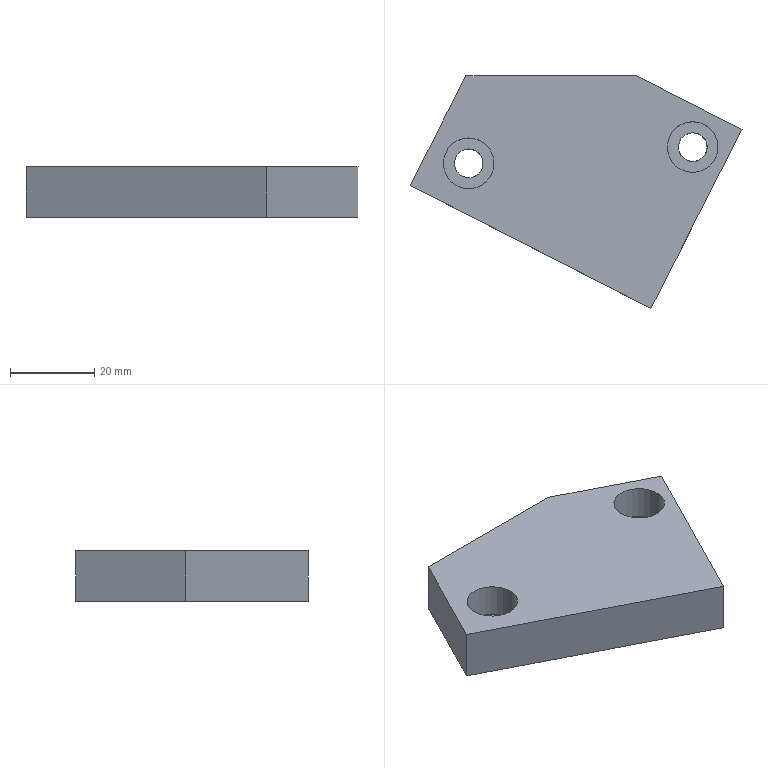Part | STEP file | gslz 2016.10.28-13_id1818_x_t | 1 solid | 13 faces | box 78.589 x 55.064 x 12 mm | volume 30432 mm3 | plane 9 | cylinder 4 | commonest cylinder face diameters 6.8 x2 12 x2
STEP:
#1=CARTESIAN_POINT('',(0.,0.,0.));
#2=DIRECTION('',(0.,0.,1.));
#3=DIRECTION('',(1.,0.,0.));
#4=AXIS2_PLACEMENT_3D('',#1,#2,#3);
#5=CARTESIAN_POINT('',(1106.682,67.903,-53.5));
#6=VERTEX_POINT('',#5);
#7=CARTESIAN_POINT('',(1081.677,80.644,-53.5));
#8=VERTEX_POINT('',#7);
#9=CARTESIAN_POINT('',(1058.568,92.419,-53.5));
#10=DIRECTION('',(-0.891,0.454,0.));
#11=VECTOR('',#10,1.);
#12=LINE('',#9,#11);
#13=CARTESIAN_POINT('',(1058.568,92.419,-29.));
#14=DIRECTION('',(0.454,0.891,0.));
#15=DIRECTION('',(-0.891,0.454,0.));
#16=AXIS2_PLACEMENT_3D('',#13,#14,#15);
#17=PLANE('',#16);
#18=CARTESIAN_POINT('',(0.,-24.5));
#19=DIRECTION('',(1.,0.));
#20=VECTOR('',#19,1.);
#21=LINE('',#18,#20);
#22=(GEOMETRIC_REPRESENTATION_CONTEXT(2)PARAMETRIC_REPRESENTATION_CONTEXT()REPRESENTATION_CONTEXT('',''));
#23=DEFINITIONAL_REPRESENTATION('',(#21),#22);
#24=PCURVE('',#17,#23);
#25=CARTESIAN_POINT('',(1068.926,57.68,-53.5));
#26=DIRECTION('',(0.,0.,1.));
#27=DIRECTION('',(1.,0.,0.));
#28=AXIS2_PLACEMENT_3D('',#25,#26,#27);
#29=PLANE('',#28);
#30=CARTESIAN_POINT('',(-10.358,34.739));
#31=DIRECTION('',(-0.891,0.454));
#32=VECTOR('',#31,1.);
#33=LINE('',#30,#32);
#34=(GEOMETRIC_REPRESENTATION_CONTEXT(2)PARAMETRIC_REPRESENTATION_CONTEXT()REPRESENTATION_CONTEXT('',''));
#35=DEFINITIONAL_REPRESENTATION('',(#33),#34);
#36=PCURVE('',#29,#35);
#37=SURFACE_CURVE('',#12,(#24,#36),.PCURVE_S1.);
#38=EDGE_CURVE('',#6,#8,#37,.T.);
#39=ORIENTED_EDGE('',*,*,#38,.T.);
#40=CARTESIAN_POINT('',(1081.677,80.644,-41.5));
#41=VERTEX_POINT('',#40);
#42=CARTESIAN_POINT('',(1081.677,80.644,-29.));
#43=DIRECTION('',(0.,0.,1.));
#44=VECTOR('',#43,1.);
#45=LINE('',#42,#44);
#46=CARTESIAN_POINT('',(-25.936,0.));
#47=DIRECTION('',(0.,1.));
#48=VECTOR('',#47,1.);
#49=LINE('',#46,#48);
#50=(GEOMETRIC_REPRESENTATION_CONTEXT(2)PARAMETRIC_REPRESENTATION_CONTEXT()REPRESENTATION_CONTEXT('',''));
#51=DEFINITIONAL_REPRESENTATION('',(#49),#50);
#52=PCURVE('',#17,#51);
#53=CARTESIAN_POINT('',(183.809,80.644,240.));
#54=DIRECTION('',(0.,1.,0.));
#55=DIRECTION('',(0.,0.,1.));
#56=AXIS2_PLACEMENT_3D('',#53,#54,#55);
#57=PLANE('',#56);
#58=CARTESIAN_POINT('',(-269.,897.868));
#59=DIRECTION('',(1.,0.));
#60=VECTOR('',#59,1.);
#61=LINE('',#58,#60);
#62=(GEOMETRIC_REPRESENTATION_CONTEXT(2)PARAMETRIC_REPRESENTATION_CONTEXT()REPRESENTATION_CONTEXT('',''));
#63=DEFINITIONAL_REPRESENTATION('',(#61),#62);
#64=PCURVE('',#57,#63);
#65=SURFACE_CURVE('',#45,(#52,#64),.PCURVE_S1.);
#66=EDGE_CURVE('',#8,#41,#65,.T.);
#67=ORIENTED_EDGE('',*,*,#66,.T.);
#68=CARTESIAN_POINT('',(1106.682,67.903,-41.5));
#69=VERTEX_POINT('',#68);
#70=CARTESIAN_POINT('',(1058.568,92.419,-41.5));
#71=DIRECTION('',(0.891,-0.454,0.));
#72=VECTOR('',#71,1.);
#73=LINE('',#70,#72);
#74=CARTESIAN_POINT('',(0.,-12.5));
#75=DIRECTION('',(-1.,0.));
#76=VECTOR('',#75,1.);
#77=LINE('',#74,#76);
#78=(GEOMETRIC_REPRESENTATION_CONTEXT(2)PARAMETRIC_REPRESENTATION_CONTEXT()REPRESENTATION_CONTEXT('',''));
#79=DEFINITIONAL_REPRESENTATION('',(#77),#78);
#80=PCURVE('',#17,#79);
#81=CARTESIAN_POINT('',(981.389,-59.052,-41.5));
#82=DIRECTION('',(0.,0.,1.));
#83=DIRECTION('',(0.,-1.,0.));
#84=AXIS2_PLACEMENT_3D('',#81,#82,#83);
#85=PLANE('',#84);
#86=CARTESIAN_POINT('',(-151.471,77.178));
#87=DIRECTION('',(0.454,0.891));
#88=VECTOR('',#87,1.);
#89=LINE('',#86,#88);
#90=(GEOMETRIC_REPRESENTATION_CONTEXT(2)PARAMETRIC_REPRESENTATION_CONTEXT()REPRESENTATION_CONTEXT('',''));
#91=DEFINITIONAL_REPRESENTATION('',(#89),#90);
#92=PCURVE('',#85,#91);
#93=SURFACE_CURVE('',#73,(#80,#92),.PCURVE_S1.);
#94=EDGE_CURVE('',#41,#69,#93,.T.);
#95=ORIENTED_EDGE('',*,*,#94,.T.);
#96=CARTESIAN_POINT('',(1106.682,67.903,-29.));
#97=DIRECTION('',(0.,0.,1.));
#98=VECTOR('',#97,1.);
#99=LINE('',#96,#98);
#100=CARTESIAN_POINT('',(-54.,0.));
#101=DIRECTION('',(0.,1.));
#102=VECTOR('',#101,1.);
#103=LINE('',#100,#102);
#104=(GEOMETRIC_REPRESENTATION_CONTEXT(2)PARAMETRIC_REPRESENTATION_CONTEXT()REPRESENTATION_CONTEXT('',''));
#105=DEFINITIONAL_REPRESENTATION('',(#103),#104);
#106=PCURVE('',#17,#105);
#107=CARTESIAN_POINT('',(1048.377,-46.527,-228.329));
#108=DIRECTION('',(-0.891,0.454,0.));
#109=DIRECTION('',(-0.000000001,-0.000000001,1.));
#110=AXIS2_PLACEMENT_3D('',#107,#108,#109);
#111=PLANE('',#110);
#112=CARTESIAN_POINT('',(199.329,128.428));
#113=DIRECTION('',(1.,0.000000001));
#114=VECTOR('',#113,1.);
#115=LINE('',#112,#114);
#116=(GEOMETRIC_REPRESENTATION_CONTEXT(2)PARAMETRIC_REPRESENTATION_CONTEXT()REPRESENTATION_CONTEXT('',''));
#117=DEFINITIONAL_REPRESENTATION('',(#115),#116);
#118=PCURVE('',#111,#117);
#119=SURFACE_CURVE('',#99,(#106,#118),.PCURVE_S1.);
#120=EDGE_CURVE('',#6,#69,#119,.T.);
#121=ORIENTED_EDGE('',*,*,#120,.F.);
#122=EDGE_LOOP('',(#39,#67,#95,#121));
#123=FACE_BOUND('',#122,.T.);
#124=ADVANCED_FACE('',(#123),#17,.T.);
#125=CARTESIAN_POINT('',(1028.093,54.636,-53.5));
#126=VERTEX_POINT('',#125);
#127=CARTESIAN_POINT('',(1085.117,25.581,-53.5));
#128=VERTEX_POINT('',#127);
#129=CARTESIAN_POINT('',(1037.003,50.096,-53.5));
#130=DIRECTION('',(0.891,-0.454,0.));
#131=VECTOR('',#130,1.);
#132=LINE('',#129,#131);
#133=CARTESIAN_POINT('',(1037.003,50.096,-228.329));
#134=DIRECTION('',(-0.454,-0.891,0.));
#135=DIRECTION('',(0.891,-0.454,0.));
#136=AXIS2_PLACEMENT_3D('',#133,#134,#135);
#137=PLANE('',#136);
#138=CARTESIAN_POINT('',(0.,174.829));
#139=DIRECTION('',(1.,0.));
#140=VECTOR('',#139,1.);
#141=LINE('',#138,#140);
#142=(GEOMETRIC_REPRESENTATION_CONTEXT(2)PARAMETRIC_REPRESENTATION_CONTEXT()REPRESENTATION_CONTEXT('',''));
#143=DEFINITIONAL_REPRESENTATION('',(#141),#142);
#144=PCURVE('',#137,#143);
#145=CARTESIAN_POINT('',(-31.922,-7.584));
#146=DIRECTION('',(0.891,-0.454));
#147=VECTOR('',#146,1.);
#148=LINE('',#145,#147);
#149=(GEOMETRIC_REPRESENTATION_CONTEXT(2)PARAMETRIC_REPRESENTATION_CONTEXT()REPRESENTATION_CONTEXT('',''));
#150=DEFINITIONAL_REPRESENTATION('',(#148),#149);
#151=PCURVE('',#29,#150);
#152=SURFACE_CURVE('',#132,(#144,#151),.PCURVE_S1.);
#153=EDGE_CURVE('',#126,#128,#152,.T.);
#154=ORIENTED_EDGE('',*,*,#153,.T.);
#155=CARTESIAN_POINT('',(1085.117,25.581,-41.5));
#156=VERTEX_POINT('',#155);
#157=CARTESIAN_POINT('',(1085.117,25.581,-228.329));
#158=DIRECTION('',(0.,0.,-1.));
#159=VECTOR('',#158,1.);
#160=LINE('',#157,#159);
#161=CARTESIAN_POINT('',(54.,0.));
#162=DIRECTION('',(0.,-1.));
#163=VECTOR('',#162,1.);
#164=LINE('',#161,#163);
#165=(GEOMETRIC_REPRESENTATION_CONTEXT(2)PARAMETRIC_REPRESENTATION_CONTEXT()REPRESENTATION_CONTEXT('',''));
#166=DEFINITIONAL_REPRESENTATION('',(#164),#165);
#167=PCURVE('',#137,#166);
#168=CARTESIAN_POINT('',(-0.000000103,80.928));
#169=DIRECTION('',(-1.,-0.000000001));
#170=VECTOR('',#169,1.);
#171=LINE('',#168,#170);
#172=(GEOMETRIC_REPRESENTATION_CONTEXT(2)PARAMETRIC_REPRESENTATION_CONTEXT()REPRESENTATION_CONTEXT('',''));
#173=DEFINITIONAL_REPRESENTATION('',(#171),#172);
#174=PCURVE('',#111,#173);
#175=SURFACE_CURVE('',#160,(#167,#174),.PCURVE_S1.);
#176=EDGE_CURVE('',#156,#128,#175,.T.);
#177=ORIENTED_EDGE('',*,*,#176,.F.);
#178=CARTESIAN_POINT('',(1028.093,54.636,-41.5));
#179=VERTEX_POINT('',#178);
#180=CARTESIAN_POINT('',(1037.003,50.096,-41.5));
#181=DIRECTION('',(0.891,-0.454,0.));
#182=VECTOR('',#181,1.);
#183=LINE('',#180,#182);
#184=CARTESIAN_POINT('',(0.,186.829));
#185=DIRECTION('',(1.,0.));
#186=VECTOR('',#185,1.);
#187=LINE('',#184,#186);
#188=(GEOMETRIC_REPRESENTATION_CONTEXT(2)PARAMETRIC_REPRESENTATION_CONTEXT()REPRESENTATION_CONTEXT('',''));
#189=DEFINITIONAL_REPRESENTATION('',(#187),#188);
#190=PCURVE('',#137,#189);
#191=CARTESIAN_POINT('',(-109.148,55.614));
#192=DIRECTION('',(0.454,0.891));
#193=VECTOR('',#192,1.);
#194=LINE('',#191,#193);
#195=(GEOMETRIC_REPRESENTATION_CONTEXT(2)PARAMETRIC_REPRESENTATION_CONTEXT()REPRESENTATION_CONTEXT('',''));
#196=DEFINITIONAL_REPRESENTATION('',(#194),#195);
#197=PCURVE('',#85,#196);
#198=SURFACE_CURVE('',#183,(#190,#197),.PCURVE_S1.);
#199=EDGE_CURVE('',#179,#156,#198,.T.);
#200=ORIENTED_EDGE('',*,*,#199,.F.);
#201=CARTESIAN_POINT('',(1028.093,54.636,-228.329));
#202=DIRECTION('',(0.,0.,-1.));
#203=VECTOR('',#202,1.);
#204=LINE('',#201,#203);
#205=CARTESIAN_POINT('',(-10.,0.));
#206=DIRECTION('',(0.,-1.));
#207=VECTOR('',#206,1.);
#208=LINE('',#205,#207);
#209=(GEOMETRIC_REPRESENTATION_CONTEXT(2)PARAMETRIC_REPRESENTATION_CONTEXT()REPRESENTATION_CONTEXT('',''));
#210=DEFINITIONAL_REPRESENTATION('',(#208),#209);
#211=PCURVE('',#137,#210);
#212=CARTESIAN_POINT('',(991.353,-17.471,-228.329));
#213=DIRECTION('',(-0.891,0.454,0.));
#214=DIRECTION('',(-0.000000001,-0.000000001,1.));
#215=AXIS2_PLACEMENT_3D('',#212,#213,#214);
#216=PLANE('',#215);
#217=CARTESIAN_POINT('',(-0.000000103,80.928));
#218=DIRECTION('',(-1.,-0.000000001));
#219=VECTOR('',#218,1.);
#220=LINE('',#217,#219);
#221=(GEOMETRIC_REPRESENTATION_CONTEXT(2)PARAMETRIC_REPRESENTATION_CONTEXT()REPRESENTATION_CONTEXT('',''));
#222=DEFINITIONAL_REPRESENTATION('',(#220),#221);
#223=PCURVE('',#216,#222);
#224=SURFACE_CURVE('',#204,(#211,#223),.PCURVE_S1.);
#225=EDGE_CURVE('',#179,#126,#224,.T.);
#226=ORIENTED_EDGE('',*,*,#225,.T.);
#227=EDGE_LOOP('',(#154,#177,#200,#226));
#228=FACE_BOUND('',#227,.T.);
#229=ADVANCED_FACE('',(#228),#137,.T.);
#230=CARTESIAN_POINT('',(1041.997,65.897,-41.5));
#231=VERTEX_POINT('',#230);
#232=CARTESIAN_POINT('',(1041.997,59.897,-41.5));
#233=DIRECTION('',(0.,0.,-1.));
#234=DIRECTION('',(0.,1.,0.));
#235=AXIS2_PLACEMENT_3D('',#232,#233,#234);
#236=CIRCLE('',#235,6.);
#237=CARTESIAN_POINT('',(-124.949,60.608));
#238=CARTESIAN_POINT('',(-124.949,71.));
#239=CARTESIAN_POINT('',(-115.949,65.804));
#240=CARTESIAN_POINT('',(-106.949,60.608));
#241=CARTESIAN_POINT('',(-115.949,55.412));
#242=CARTESIAN_POINT('',(-124.949,50.215));
#243=CARTESIAN_POINT('',(-124.949,60.608));
#244=(BOUNDED_CURVE()B_SPLINE_CURVE(2,(#237,#238,#239,#240,#241,#242,#243),.UNSPECIFIED.,.T.,.F.)B_SPLINE_CURVE_WITH_KNOTS((1,2,2,2,2,1),(-2.094,0.,2.094,4.189,6.283,8.378),.UNSPECIFIED.)CURVE()GEOMETRIC_REPRESENTATION_ITEM()RATIONAL_B_SPLINE_CURVE((1.,0.5,1.,0.5,1.,0.5,1.))REPRESENTATION_ITEM(''));
#245=(GEOMETRIC_REPRESENTATION_CONTEXT(2)PARAMETRIC_REPRESENTATION_CONTEXT()REPRESENTATION_CONTEXT('',''));
#246=DEFINITIONAL_REPRESENTATION('',(#244),#245);
#247=PCURVE('',#85,#246);
#248=CARTESIAN_POINT('',(1041.997,59.897,-41.5));
#249=DIRECTION('',(0.,0.,-1.));
#250=DIRECTION('',(0.,1.,0.));
#251=AXIS2_PLACEMENT_3D('',#248,#249,#250);
#252=CYLINDRICAL_SURFACE('',#251,6.);
#253=CARTESIAN_POINT('',(0.,0.));
#254=DIRECTION('',(1.,0.));
#255=VECTOR('',#254,1.);
#256=LINE('',#253,#255);
#257=(GEOMETRIC_REPRESENTATION_CONTEXT(2)PARAMETRIC_REPRESENTATION_CONTEXT()REPRESENTATION_CONTEXT('',''));
#258=DEFINITIONAL_REPRESENTATION('',(#256),#257);
#259=PCURVE('',#252,#258);
#260=SURFACE_CURVE('',#236,(#247,#259),.PCURVE_S1.);
#261=EDGE_CURVE('',#231,#231,#260,.T.);
#262=ORIENTED_EDGE('',*,*,#261,.T.);
#263=EDGE_LOOP('',(#262));
#264=FACE_BOUND('',#263,.T.);
#265=CARTESIAN_POINT('',(1095.023,69.743,-41.5));
#266=VERTEX_POINT('',#265);
#267=CARTESIAN_POINT('',(1095.023,63.743,-41.5));
#268=DIRECTION('',(0.,0.,-1.));
#269=DIRECTION('',(0.,1.,0.));
#270=AXIS2_PLACEMENT_3D('',#267,#268,#269);
#271=CIRCLE('',#270,6.);
#272=CARTESIAN_POINT('',(-128.795,113.633));
#273=CARTESIAN_POINT('',(-128.795,124.026));
#274=CARTESIAN_POINT('',(-119.795,118.829));
#275=CARTESIAN_POINT('',(-110.795,113.633));
#276=CARTESIAN_POINT('',(-119.795,108.437));
#277=CARTESIAN_POINT('',(-128.795,103.241));
#278=CARTESIAN_POINT('',(-128.795,113.633));
#279=(BOUNDED_CURVE()B_SPLINE_CURVE(2,(#272,#273,#274,#275,#276,#277,#278),.UNSPECIFIED.,.T.,.F.)B_SPLINE_CURVE_WITH_KNOTS((1,2,2,2,2,1),(-2.094,0.,2.094,4.189,6.283,8.378),.UNSPECIFIED.)CURVE()GEOMETRIC_REPRESENTATION_ITEM()RATIONAL_B_SPLINE_CURVE((1.,0.5,1.,0.5,1.,0.5,1.))REPRESENTATION_ITEM(''));
#280=(GEOMETRIC_REPRESENTATION_CONTEXT(2)PARAMETRIC_REPRESENTATION_CONTEXT()REPRESENTATION_CONTEXT('',''));
#281=DEFINITIONAL_REPRESENTATION('',(#279),#280);
#282=PCURVE('',#85,#281);
#283=CARTESIAN_POINT('',(1095.023,63.743,-41.5));
#284=DIRECTION('',(0.,0.,-1.));
#285=DIRECTION('',(0.,1.,0.));
#286=AXIS2_PLACEMENT_3D('',#283,#284,#285);
#287=CYLINDRICAL_SURFACE('',#286,6.);
#288=CARTESIAN_POINT('',(0.,0.));
#289=DIRECTION('',(1.,0.));
#290=VECTOR('',#289,1.);
#291=LINE('',#288,#290);
#292=(GEOMETRIC_REPRESENTATION_CONTEXT(2)PARAMETRIC_REPRESENTATION_CONTEXT()REPRESENTATION_CONTEXT('',''));
#293=DEFINITIONAL_REPRESENTATION('',(#291),#292);
#294=PCURVE('',#287,#293);
#295=SURFACE_CURVE('',#271,(#282,#294),.PCURVE_S1.);
#296=EDGE_CURVE('',#266,#266,#295,.T.);
#297=ORIENTED_EDGE('',*,*,#296,.T.);
#298=EDGE_LOOP('',(#297));
#299=FACE_BOUND('',#298,.T.);
#300=ORIENTED_EDGE('',*,*,#94,.F.);
#301=CARTESIAN_POINT('',(1041.345,80.644,-41.5));
#302=VERTEX_POINT('',#301);
#303=CARTESIAN_POINT('',(981.389,80.644,-41.5));
#304=DIRECTION('',(-1.,0.,0.));
#305=VECTOR('',#304,1.);
#306=LINE('',#303,#305);
#307=CARTESIAN_POINT('',(-139.696,0.));
#308=DIRECTION('',(0.,-1.));
#309=VECTOR('',#308,1.);
#310=LINE('',#307,#309);
#311=(GEOMETRIC_REPRESENTATION_CONTEXT(2)PARAMETRIC_REPRESENTATION_CONTEXT()REPRESENTATION_CONTEXT('',''));
#312=DEFINITIONAL_REPRESENTATION('',(#310),#311);
#313=PCURVE('',#85,#312);
#314=CARTESIAN_POINT('',(-281.5,797.58));
#315=DIRECTION('',(0.,-1.));
#316=VECTOR('',#315,1.);
#317=LINE('',#314,#316);
#318=(GEOMETRIC_REPRESENTATION_CONTEXT(2)PARAMETRIC_REPRESENTATION_CONTEXT()REPRESENTATION_CONTEXT('',''));
#319=DEFINITIONAL_REPRESENTATION('',(#317),#318);
#320=PCURVE('',#57,#319);
#321=SURFACE_CURVE('',#306,(#313,#320),.PCURVE_S1.);
#322=EDGE_CURVE('',#41,#302,#321,.T.);
#323=ORIENTED_EDGE('',*,*,#322,.T.);
#324=CARTESIAN_POINT('',(972.479,-54.512,-41.5));
#325=DIRECTION('',(0.454,0.891,0.));
#326=VECTOR('',#325,1.);
#327=LINE('',#324,#326);
#328=CARTESIAN_POINT('',(-4.54,-8.91));
#329=DIRECTION('',(-0.891,0.454));
#330=VECTOR('',#329,1.);
#331=LINE('',#328,#330);
#332=(GEOMETRIC_REPRESENTATION_CONTEXT(2)PARAMETRIC_REPRESENTATION_CONTEXT()REPRESENTATION_CONTEXT('',''));
#333=DEFINITIONAL_REPRESENTATION('',(#331),#332);
#334=PCURVE('',#85,#333);
#335=CARTESIAN_POINT('',(186.829,-41.572));
#336=DIRECTION('',(-0.000000001,1.));
#337=VECTOR('',#336,1.);
#338=LINE('',#335,#337);
#339=(GEOMETRIC_REPRESENTATION_CONTEXT(2)PARAMETRIC_REPRESENTATION_CONTEXT()REPRESENTATION_CONTEXT('',''));
#340=DEFINITIONAL_REPRESENTATION('',(#338),#339);
#341=PCURVE('',#216,#340);
#342=SURFACE_CURVE('',#327,(#334,#341),.PCURVE_S1.);
#343=EDGE_CURVE('',#179,#302,#342,.T.);
#344=ORIENTED_EDGE('',*,*,#343,.F.);
#345=ORIENTED_EDGE('',*,*,#199,.T.);
#346=CARTESIAN_POINT('',(1029.504,-83.568,-41.5));
#347=DIRECTION('',(0.454,0.891,0.));
#348=VECTOR('',#347,1.);
#349=LINE('',#346,#348);
#350=CARTESIAN_POINT('',(24.515,48.114));
#351=DIRECTION('',(-0.891,0.454));
#352=VECTOR('',#351,1.);
#353=LINE('',#350,#352);
#354=(GEOMETRIC_REPRESENTATION_CONTEXT(2)PARAMETRIC_REPRESENTATION_CONTEXT()REPRESENTATION_CONTEXT('',''));
#355=DEFINITIONAL_REPRESENTATION('',(#353),#354);
#356=PCURVE('',#85,#355);
#357=CARTESIAN_POINT('',(186.829,-41.572));
#358=DIRECTION('',(-0.000000001,1.));
#359=VECTOR('',#358,1.);
#360=LINE('',#357,#359);
#361=(GEOMETRIC_REPRESENTATION_CONTEXT(2)PARAMETRIC_REPRESENTATION_CONTEXT()REPRESENTATION_CONTEXT('',''));
#362=DEFINITIONAL_REPRESENTATION('',(#360),#361);
#363=PCURVE('',#111,#362);
#364=SURFACE_CURVE('',#349,(#356,#363),.PCURVE_S1.);
#365=EDGE_CURVE('',#156,#69,#364,.T.);
#366=ORIENTED_EDGE('',*,*,#365,.T.);
#367=EDGE_LOOP('',(#300,#323,#344,#345,#366));
#368=FACE_BOUND('',#367,.T.);
#369=ADVANCED_FACE('',(#264,#299,#368),#85,.T.);
#370=ORIENTED_EDGE('',*,*,#343,.T.);
#371=CARTESIAN_POINT('',(1041.345,80.644,-53.5));
#372=VERTEX_POINT('',#371);
#373=CARTESIAN_POINT('',(1041.345,80.644,240.));
#374=DIRECTION('',(0.,0.,-1.));
#375=VECTOR('',#374,1.);
#376=LINE('',#373,#375);
#377=CARTESIAN_POINT('',(468.329,110.118));
#378=DIRECTION('',(-1.,-0.000000001));
#379=VECTOR('',#378,1.);
#380=LINE('',#377,#379);
#381=(GEOMETRIC_REPRESENTATION_CONTEXT(2)PARAMETRIC_REPRESENTATION_CONTEXT()REPRESENTATION_CONTEXT('',''));
#382=DEFINITIONAL_REPRESENTATION('',(#380),#381);
#383=PCURVE('',#216,#382);
#384=CARTESIAN_POINT('',(0.,857.536));
#385=DIRECTION('',(-1.,0.));
#386=VECTOR('',#385,1.);
#387=LINE('',#384,#386);
#388=(GEOMETRIC_REPRESENTATION_CONTEXT(2)PARAMETRIC_REPRESENTATION_CONTEXT()REPRESENTATION_CONTEXT('',''));
#389=DEFINITIONAL_REPRESENTATION('',(#387),#388);
#390=PCURVE('',#57,#389);
#391=SURFACE_CURVE('',#376,(#383,#390),.PCURVE_S1.);
#392=EDGE_CURVE('',#302,#372,#391,.T.);
#393=ORIENTED_EDGE('',*,*,#392,.T.);
#394=CARTESIAN_POINT('',(991.353,-17.471,-53.5));
#395=DIRECTION('',(0.454,0.891,0.));
#396=VECTOR('',#395,1.);
#397=LINE('',#394,#396);
#398=CARTESIAN_POINT('',(174.829,0.000000222));
#399=DIRECTION('',(-0.000000001,1.));
#400=VECTOR('',#399,1.);
#401=LINE('',#398,#400);
#402=(GEOMETRIC_REPRESENTATION_CONTEXT(2)PARAMETRIC_REPRESENTATION_CONTEXT()REPRESENTATION_CONTEXT('',''));
#403=DEFINITIONAL_REPRESENTATION('',(#401),#402);
#404=PCURVE('',#216,#403);
#405=CARTESIAN_POINT('',(-77.573,-75.152));
#406=DIRECTION('',(0.454,0.891));
#407=VECTOR('',#406,1.);
#408=LINE('',#405,#407);
#409=(GEOMETRIC_REPRESENTATION_CONTEXT(2)PARAMETRIC_REPRESENTATION_CONTEXT()REPRESENTATION_CONTEXT('',''));
#410=DEFINITIONAL_REPRESENTATION('',(#408),#409);
#411=PCURVE('',#29,#410);
#412=SURFACE_CURVE('',#397,(#404,#411),.PCURVE_S1.);
#413=EDGE_CURVE('',#126,#372,#412,.T.);
#414=ORIENTED_EDGE('',*,*,#413,.F.);
#415=ORIENTED_EDGE('',*,*,#225,.F.);
#416=EDGE_LOOP('',(#370,#393,#414,#415));
#417=FACE_BOUND('',#416,.T.);
#418=ADVANCED_FACE('',(#417),#216,.T.);
#419=CARTESIAN_POINT('',(1048.377,-46.527,-53.5));
#420=DIRECTION('',(-0.454,-0.891,0.));
#421=VECTOR('',#420,1.);
#422=LINE('',#419,#421);
#423=CARTESIAN_POINT('',(174.829,0.000000222));
#424=DIRECTION('',(0.000000001,-1.));
#425=VECTOR('',#424,1.);
#426=LINE('',#423,#425);
#427=(GEOMETRIC_REPRESENTATION_CONTEXT(2)PARAMETRIC_REPRESENTATION_CONTEXT()REPRESENTATION_CONTEXT('',''));
#428=DEFINITIONAL_REPRESENTATION('',(#426),#427);
#429=PCURVE('',#111,#428);
#430=CARTESIAN_POINT('',(-20.549,-104.207));
#431=DIRECTION('',(-0.454,-0.891));
#432=VECTOR('',#431,1.);
#433=LINE('',#430,#432);
#434=(GEOMETRIC_REPRESENTATION_CONTEXT(2)PARAMETRIC_REPRESENTATION_CONTEXT()REPRESENTATION_CONTEXT('',''));
#435=DEFINITIONAL_REPRESENTATION('',(#433),#434);
#436=PCURVE('',#29,#435);
#437=SURFACE_CURVE('',#422,(#429,#436),.PCURVE_S1.);
#438=EDGE_CURVE('',#6,#128,#437,.T.);
#439=ORIENTED_EDGE('',*,*,#438,.F.);
#440=ORIENTED_EDGE('',*,*,#120,.T.);
#441=ORIENTED_EDGE('',*,*,#365,.F.);
#442=ORIENTED_EDGE('',*,*,#176,.T.);
#443=EDGE_LOOP('',(#439,#440,#441,#442));
#444=FACE_BOUND('',#443,.T.);
#445=ADVANCED_FACE('',(#444),#111,.F.);
#446=CARTESIAN_POINT('',(1045.397,59.897,-53.5));
#447=VERTEX_POINT('',#446);
#448=CARTESIAN_POINT('',(1041.997,63.297,-53.5));
#449=VERTEX_POINT('',#448);
#450=CARTESIAN_POINT('',(1041.997,59.897,-53.5));
#451=DIRECTION('',(0.,0.,1.));
#452=DIRECTION('',(1.,0.,0.));
#453=AXIS2_PLACEMENT_3D('',#450,#451,#452);
#454=CIRCLE('',#453,3.4);
#455=CARTESIAN_POINT('',(-26.929,2.217));
#456=DIRECTION('',(1.,0.));
#457=AXIS2_PLACEMENT_2D('',#455,#456);
#458=CIRCLE('',#457,3.4);
#459=(GEOMETRIC_REPRESENTATION_CONTEXT(2)PARAMETRIC_REPRESENTATION_CONTEXT()REPRESENTATION_CONTEXT('',''));
#460=DEFINITIONAL_REPRESENTATION('',(#458),#459);
#461=PCURVE('',#29,#460);
#462=CARTESIAN_POINT('',(1041.997,59.897,-91.5));
#463=DIRECTION('',(0.,0.,-1.));
#464=DIRECTION('',(0.,1.,0.));
#465=AXIS2_PLACEMENT_3D('',#462,#463,#464);
#466=CYLINDRICAL_SURFACE('',#465,3.4);
#467=CARTESIAN_POINT('',(1.571,-38.));
#468=DIRECTION('',(-1.,0.));
#469=VECTOR('',#468,1.);
#470=LINE('',#467,#469);
#471=(GEOMETRIC_REPRESENTATION_CONTEXT(2)PARAMETRIC_REPRESENTATION_CONTEXT()REPRESENTATION_CONTEXT('',''));
#472=DEFINITIONAL_REPRESENTATION('',(#470),#471);
#473=PCURVE('',#466,#472);
#474=SURFACE_CURVE('',#454,(#461,#473),.PCURVE_S1.);
#475=EDGE_CURVE('',#447,#449,#474,.T.);
#476=ORIENTED_EDGE('',*,*,#475,.T.);
#477=CARTESIAN_POINT('',(1041.997,59.897,-53.5));
#478=DIRECTION('',(0.,0.,1.));
#479=DIRECTION('',(1.,0.,0.));
#480=AXIS2_PLACEMENT_3D('',#477,#478,#479);
#481=CIRCLE('',#480,3.4);
#482=CARTESIAN_POINT('',(-26.929,2.217));
#483=DIRECTION('',(1.,0.));
#484=AXIS2_PLACEMENT_2D('',#482,#483);
#485=CIRCLE('',#484,3.4);
#486=(GEOMETRIC_REPRESENTATION_CONTEXT(2)PARAMETRIC_REPRESENTATION_CONTEXT()REPRESENTATION_CONTEXT('',''));
#487=DEFINITIONAL_REPRESENTATION('',(#485),#486);
#488=PCURVE('',#29,#487);
#489=CARTESIAN_POINT('',(7.854,-38.));
#490=DIRECTION('',(-1.,0.));
#491=VECTOR('',#490,1.);
#492=LINE('',#489,#491);
#493=(GEOMETRIC_REPRESENTATION_CONTEXT(2)PARAMETRIC_REPRESENTATION_CONTEXT()REPRESENTATION_CONTEXT('',''));
#494=DEFINITIONAL_REPRESENTATION('',(#492),#493);
#495=PCURVE('',#466,#494);
#496=SURFACE_CURVE('',#481,(#488,#495),.PCURVE_S1.);
#497=EDGE_CURVE('',#449,#447,#496,.T.);
#498=ORIENTED_EDGE('',*,*,#497,.T.);
#499=EDGE_LOOP('',(#476,#498));
#500=FACE_BOUND('',#499,.T.);
#501=CARTESIAN_POINT('',(1098.423,63.743,-53.5));
#502=VERTEX_POINT('',#501);
#503=CARTESIAN_POINT('',(1095.023,67.143,-53.5));
#504=VERTEX_POINT('',#503);
#505=CARTESIAN_POINT('',(1095.023,63.743,-53.5));
#506=DIRECTION('',(0.,0.,1.));
#507=DIRECTION('',(1.,0.,0.));
#508=AXIS2_PLACEMENT_3D('',#505,#506,#507);
#509=CIRCLE('',#508,3.4);
#510=CARTESIAN_POINT('',(26.097,6.063));
#511=DIRECTION('',(1.,0.));
#512=AXIS2_PLACEMENT_2D('',#510,#511);
#513=CIRCLE('',#512,3.4);
#514=(GEOMETRIC_REPRESENTATION_CONTEXT(2)PARAMETRIC_REPRESENTATION_CONTEXT()REPRESENTATION_CONTEXT('',''));
#515=DEFINITIONAL_REPRESENTATION('',(#513),#514);
#516=PCURVE('',#29,#515);
#517=CARTESIAN_POINT('',(1095.023,63.743,-91.5));
#518=DIRECTION('',(0.,0.,-1.));
#519=DIRECTION('',(0.,1.,0.));
#520=AXIS2_PLACEMENT_3D('',#517,#518,#519);
#521=CYLINDRICAL_SURFACE('',#520,3.4);
#522=CARTESIAN_POINT('',(1.571,-38.));
#523=DIRECTION('',(-1.,0.));
#524=VECTOR('',#523,1.);
#525=LINE('',#522,#524);
#526=(GEOMETRIC_REPRESENTATION_CONTEXT(2)PARAMETRIC_REPRESENTATION_CONTEXT()REPRESENTATION_CONTEXT('',''));
#527=DEFINITIONAL_REPRESENTATION('',(#525),#526);
#528=PCURVE('',#521,#527);
#529=SURFACE_CURVE('',#509,(#516,#528),.PCURVE_S1.);
#530=EDGE_CURVE('',#502,#504,#529,.T.);
#531=ORIENTED_EDGE('',*,*,#530,.T.);
#532=CARTESIAN_POINT('',(1095.023,63.743,-53.5));
#533=DIRECTION('',(0.,0.,1.));
#534=DIRECTION('',(1.,0.,0.));
#535=AXIS2_PLACEMENT_3D('',#532,#533,#534);
#536=CIRCLE('',#535,3.4);
#537=CARTESIAN_POINT('',(26.097,6.063));
#538=DIRECTION('',(1.,0.));
#539=AXIS2_PLACEMENT_2D('',#537,#538);
#540=CIRCLE('',#539,3.4);
#541=(GEOMETRIC_REPRESENTATION_CONTEXT(2)PARAMETRIC_REPRESENTATION_CONTEXT()REPRESENTATION_CONTEXT('',''));
#542=DEFINITIONAL_REPRESENTATION('',(#540),#541);
#543=PCURVE('',#29,#542);
#544=CARTESIAN_POINT('',(7.854,-38.));
#545=DIRECTION('',(-1.,0.));
#546=VECTOR('',#545,1.);
#547=LINE('',#544,#546);
#548=(GEOMETRIC_REPRESENTATION_CONTEXT(2)PARAMETRIC_REPRESENTATION_CONTEXT()REPRESENTATION_CONTEXT('',''));
#549=DEFINITIONAL_REPRESENTATION('',(#547),#548);
#550=PCURVE('',#521,#549);
#551=SURFACE_CURVE('',#536,(#543,#550),.PCURVE_S1.);
#552=EDGE_CURVE('',#504,#502,#551,.T.);
#553=ORIENTED_EDGE('',*,*,#552,.T.);
#554=EDGE_LOOP('',(#531,#553));
#555=FACE_BOUND('',#554,.T.);
#556=ORIENTED_EDGE('',*,*,#413,.T.);
#557=CARTESIAN_POINT('',(183.809,80.644,-53.5));
#558=DIRECTION('',(1.,0.,0.));
#559=VECTOR('',#558,1.);
#560=LINE('',#557,#559);
#561=CARTESIAN_POINT('',(-885.116,22.964));
#562=DIRECTION('',(1.,0.));
#563=VECTOR('',#562,1.);
#564=LINE('',#561,#563);
#565=(GEOMETRIC_REPRESENTATION_CONTEXT(2)PARAMETRIC_REPRESENTATION_CONTEXT()REPRESENTATION_CONTEXT('',''));
#566=DEFINITIONAL_REPRESENTATION('',(#564),#565);
#567=PCURVE('',#29,#566);
#568=CARTESIAN_POINT('',(-293.5,0.));
#569=DIRECTION('',(0.,1.));
#570=VECTOR('',#569,1.);
#571=LINE('',#568,#570);
#572=(GEOMETRIC_REPRESENTATION_CONTEXT(2)PARAMETRIC_REPRESENTATION_CONTEXT()REPRESENTATION_CONTEXT('',''));
#573=DEFINITIONAL_REPRESENTATION('',(#571),#572);
#574=PCURVE('',#57,#573);
#575=SURFACE_CURVE('',#560,(#567,#574),.PCURVE_S1.);
#576=EDGE_CURVE('',#372,#8,#575,.T.);
#577=ORIENTED_EDGE('',*,*,#576,.T.);
#578=ORIENTED_EDGE('',*,*,#38,.F.);
#579=ORIENTED_EDGE('',*,*,#438,.T.);
#580=ORIENTED_EDGE('',*,*,#153,.F.);
#581=EDGE_LOOP('',(#556,#577,#578,#579,#580));
#582=FACE_BOUND('',#581,.T.);
#583=ADVANCED_FACE('',(#500,#555,#582),#29,.F.);
#584=ORIENTED_EDGE('',*,*,#576,.F.);
#585=ORIENTED_EDGE('',*,*,#392,.F.);
#586=ORIENTED_EDGE('',*,*,#322,.F.);
#587=ORIENTED_EDGE('',*,*,#66,.F.);
#588=EDGE_LOOP('',(#584,#585,#586,#587));
#589=FACE_BOUND('',#588,.T.);
#590=ADVANCED_FACE('',(#589),#57,.T.);
#591=CARTESIAN_POINT('',(1095.023,67.143,-49.5));
#592=VERTEX_POINT('',#591);
#593=CARTESIAN_POINT('',(1095.023,63.743,-49.5));
#594=DIRECTION('',(0.,0.,1.));
#595=DIRECTION('',(0.,1.,0.));
#596=AXIS2_PLACEMENT_3D('',#593,#594,#595);
#597=CIRCLE('',#596,3.4);
#598=CARTESIAN_POINT('',(6.283,-42.));
#599=DIRECTION('',(-1.,0.));
#600=VECTOR('',#599,1.);
#601=LINE('',#598,#600);
#602=(GEOMETRIC_REPRESENTATION_CONTEXT(2)PARAMETRIC_REPRESENTATION_CONTEXT()REPRESENTATION_CONTEXT('',''));
#603=DEFINITIONAL_REPRESENTATION('',(#601),#602);
#604=PCURVE('',#521,#603);
#605=CARTESIAN_POINT('',(1093.661,61.07,-49.5));
#606=DIRECTION('',(0.,0.,-1.));
#607=DIRECTION('',(0.,1.,0.));
#608=AXIS2_PLACEMENT_3D('',#605,#606,#607);
#609=PLANE('',#608);
#610=CARTESIAN_POINT('',(6.073,1.362));
#611=CARTESIAN_POINT('',(6.073,-4.527));
#612=CARTESIAN_POINT('',(0.973,-1.583));
#613=CARTESIAN_POINT('',(-4.127,1.362));
#614=CARTESIAN_POINT('',(0.973,4.306));
#615=CARTESIAN_POINT('',(6.073,7.251));
#616=CARTESIAN_POINT('',(6.073,1.362));
#617=(BOUNDED_CURVE()B_SPLINE_CURVE(2,(#610,#611,#612,#613,#614,#615,#616),.UNSPECIFIED.,.T.,.F.)B_SPLINE_CURVE_WITH_KNOTS((1,2,2,2,2,1),(-2.094,0.,2.094,4.189,6.283,8.378),.UNSPECIFIED.)CURVE()GEOMETRIC_REPRESENTATION_ITEM()RATIONAL_B_SPLINE_CURVE((1.,0.5,1.,0.5,1.,0.5,1.))REPRESENTATION_ITEM(''));
#618=(GEOMETRIC_REPRESENTATION_CONTEXT(2)PARAMETRIC_REPRESENTATION_CONTEXT()REPRESENTATION_CONTEXT('',''));
#619=DEFINITIONAL_REPRESENTATION('',(#617),#618);
#620=PCURVE('',#609,#619);
#621=SURFACE_CURVE('',#597,(#604,#620),.PCURVE_S1.);
#622=EDGE_CURVE('',#592,#592,#621,.T.);
#623=ORIENTED_EDGE('',*,*,#622,.F.);
#624=CARTESIAN_POINT('',(1095.023,67.143,-49.5));
#625=CARTESIAN_POINT('',(1095.023,67.143,-53.5));
#626=B_SPLINE_CURVE_WITH_KNOTS('',1,(#624,#625),.UNSPECIFIED.,.F.,.F.,(2,2),(-42.,-38.),.PIECEWISE_BEZIER_KNOTS.);
#627=CARTESIAN_POINT('',(6.283,0.));
#628=DIRECTION('',(0.,1.));
#629=VECTOR('',#628,1.);
#630=LINE('',#627,#629);
#631=(GEOMETRIC_REPRESENTATION_CONTEXT(2)PARAMETRIC_REPRESENTATION_CONTEXT()REPRESENTATION_CONTEXT('',''));
#632=DEFINITIONAL_REPRESENTATION('',(#630),#631);
#633=PCURVE('',#521,#632);
#634=CARTESIAN_POINT('',(0.,0.));
#635=DIRECTION('',(0.,1.));
#636=VECTOR('',#635,1.);
#637=LINE('',#634,#636);
#638=(GEOMETRIC_REPRESENTATION_CONTEXT(2)PARAMETRIC_REPRESENTATION_CONTEXT()REPRESENTATION_CONTEXT('',''));
#639=DEFINITIONAL_REPRESENTATION('',(#637),#638);
#640=PCURVE('',#521,#639);
#641=SEAM_CURVE('',#626,(#633,#640),.PCURVE_S1.);
#642=EDGE_CURVE('',#592,#504,#641,.T.);
#643=ORIENTED_EDGE('',*,*,#642,.T.);
#644=ORIENTED_EDGE('',*,*,#552,.T.);
#645=ORIENTED_EDGE('',*,*,#530,.T.);
#646=ORIENTED_EDGE('',*,*,#642,.F.);
#647=EDGE_LOOP('',(#623,#643,#644,#645,#646));
#648=FACE_BOUND('',#647,.F.);
#649=ADVANCED_FACE('',(#648),#521,.F.);
#650=ORIENTED_EDGE('',*,*,#622,.F.);
#651=EDGE_LOOP('',(#650));
#652=FACE_BOUND('',#651,.T.);
#653=CARTESIAN_POINT('',(1095.023,69.743,-49.5));
#654=VERTEX_POINT('',#653);
#655=CARTESIAN_POINT('',(1095.023,63.743,-49.5));
#656=DIRECTION('',(0.,0.,1.));
#657=DIRECTION('',(0.,1.,0.));
#658=AXIS2_PLACEMENT_3D('',#655,#656,#657);
#659=CIRCLE('',#658,6.);
#660=CARTESIAN_POINT('',(8.673,1.362));
#661=CARTESIAN_POINT('',(8.673,-9.03));
#662=CARTESIAN_POINT('',(-0.327,-3.834));
#663=CARTESIAN_POINT('',(-9.327,1.362));
#664=CARTESIAN_POINT('',(-0.327,6.558));
#665=CARTESIAN_POINT('',(8.673,11.754));
#666=CARTESIAN_POINT('',(8.673,1.362));
#667=(BOUNDED_CURVE()B_SPLINE_CURVE(2,(#660,#661,#662,#663,#664,#665,#666),.UNSPECIFIED.,.T.,.F.)B_SPLINE_CURVE_WITH_KNOTS((1,2,2,2,2,1),(-2.094,0.,2.094,4.189,6.283,8.378),.UNSPECIFIED.)CURVE()GEOMETRIC_REPRESENTATION_ITEM()RATIONAL_B_SPLINE_CURVE((1.,0.5,1.,0.5,1.,0.5,1.))REPRESENTATION_ITEM(''));
#668=(GEOMETRIC_REPRESENTATION_CONTEXT(2)PARAMETRIC_REPRESENTATION_CONTEXT()REPRESENTATION_CONTEXT('',''));
#669=DEFINITIONAL_REPRESENTATION('',(#667),#668);
#670=PCURVE('',#609,#669);
#671=CARTESIAN_POINT('',(6.283,8.));
#672=DIRECTION('',(-1.,0.));
#673=VECTOR('',#672,1.);
#674=LINE('',#671,#673);
#675=(GEOMETRIC_REPRESENTATION_CONTEXT(2)PARAMETRIC_REPRESENTATION_CONTEXT()REPRESENTATION_CONTEXT('',''));
#676=DEFINITIONAL_REPRESENTATION('',(#674),#675);
#677=PCURVE('',#287,#676);
#678=SURFACE_CURVE('',#659,(#670,#677),.PCURVE_S1.);
#679=EDGE_CURVE('',#654,#654,#678,.T.);
#680=ORIENTED_EDGE('',*,*,#679,.T.);
#681=EDGE_LOOP('',(#680));
#682=FACE_BOUND('',#681,.T.);
#683=ADVANCED_FACE('',(#652,#682),#609,.F.);
#684=ORIENTED_EDGE('',*,*,#679,.T.);
#685=CARTESIAN_POINT('',(1095.023,69.743,-41.5));
#686=CARTESIAN_POINT('',(1095.023,69.743,-49.5));
#687=B_SPLINE_CURVE_WITH_KNOTS('',1,(#685,#686),.UNSPECIFIED.,.F.,.F.,(2,2),(0.,8.),.PIECEWISE_BEZIER_KNOTS.);
#688=CARTESIAN_POINT('',(0.,0.));
#689=DIRECTION('',(0.,1.));
#690=VECTOR('',#689,1.);
#691=LINE('',#688,#690);
#692=(GEOMETRIC_REPRESENTATION_CONTEXT(2)PARAMETRIC_REPRESENTATION_CONTEXT()REPRESENTATION_CONTEXT('',''));
#693=DEFINITIONAL_REPRESENTATION('',(#691),#692);
#694=PCURVE('',#287,#693);
#695=CARTESIAN_POINT('',(6.283,0.));
#696=DIRECTION('',(0.,1.));
#697=VECTOR('',#696,1.);
#698=LINE('',#695,#697);
#699=(GEOMETRIC_REPRESENTATION_CONTEXT(2)PARAMETRIC_REPRESENTATION_CONTEXT()REPRESENTATION_CONTEXT('',''));
#700=DEFINITIONAL_REPRESENTATION('',(#698),#699);
#701=PCURVE('',#287,#700);
#702=SEAM_CURVE('',#687,(#694,#701),.PCURVE_S1.);
#703=EDGE_CURVE('',#266,#654,#702,.T.);
#704=ORIENTED_EDGE('',*,*,#703,.F.);
#705=ORIENTED_EDGE('',*,*,#296,.T.);
#706=ORIENTED_EDGE('',*,*,#703,.T.);
#707=EDGE_LOOP('',(#684,#704,#705,#706));
#708=FACE_BOUND('',#707,.F.);
#709=ADVANCED_FACE('',(#708),#287,.F.);
#710=CARTESIAN_POINT('',(1041.997,63.297,-49.5));
#711=VERTEX_POINT('',#710);
#712=CARTESIAN_POINT('',(1041.997,59.897,-49.5));
#713=DIRECTION('',(0.,0.,1.));
#714=DIRECTION('',(0.,1.,0.));
#715=AXIS2_PLACEMENT_3D('',#712,#713,#714);
#716=CIRCLE('',#715,3.4);
#717=CARTESIAN_POINT('',(6.283,-42.));
#718=DIRECTION('',(-1.,0.));
#719=VECTOR('',#718,1.);
#720=LINE('',#717,#719);
#721=(GEOMETRIC_REPRESENTATION_CONTEXT(2)PARAMETRIC_REPRESENTATION_CONTEXT()REPRESENTATION_CONTEXT('',''));
#722=DEFINITIONAL_REPRESENTATION('',(#720),#721);
#723=PCURVE('',#466,#722);
#724=CARTESIAN_POINT('',(1041.997,59.897,-49.5));
#725=DIRECTION('',(0.,0.,-1.));
#726=DIRECTION('',(0.,1.,0.));
#727=AXIS2_PLACEMENT_3D('',#724,#725,#726);
#728=PLANE('',#727);
#729=CARTESIAN_POINT('',(3.4,0.));
#730=CARTESIAN_POINT('',(3.4,-5.889));
#731=CARTESIAN_POINT('',(-1.7,-2.944));
#732=CARTESIAN_POINT('',(-6.8,0.));
#733=CARTESIAN_POINT('',(-1.7,2.944));
#734=CARTESIAN_POINT('',(3.4,5.889));
#735=CARTESIAN_POINT('',(3.4,0.));
#736=(BOUNDED_CURVE()B_SPLINE_CURVE(2,(#729,#730,#731,#732,#733,#734,#735),.UNSPECIFIED.,.T.,.F.)B_SPLINE_CURVE_WITH_KNOTS((1,2,2,2,2,1),(-2.094,0.,2.094,4.189,6.283,8.378),.UNSPECIFIED.)CURVE()GEOMETRIC_REPRESENTATION_ITEM()RATIONAL_B_SPLINE_CURVE((1.,0.5,1.,0.5,1.,0.5,1.))REPRESENTATION_ITEM(''));
#737=(GEOMETRIC_REPRESENTATION_CONTEXT(2)PARAMETRIC_REPRESENTATION_CONTEXT()REPRESENTATION_CONTEXT('',''));
#738=DEFINITIONAL_REPRESENTATION('',(#736),#737);
#739=PCURVE('',#728,#738);
#740=SURFACE_CURVE('',#716,(#723,#739),.PCURVE_S1.);
#741=EDGE_CURVE('',#711,#711,#740,.T.);
#742=ORIENTED_EDGE('',*,*,#741,.F.);
#743=CARTESIAN_POINT('',(1041.997,63.297,-49.5));
#744=CARTESIAN_POINT('',(1041.997,63.297,-53.5));
#745=B_SPLINE_CURVE_WITH_KNOTS('',1,(#743,#744),.UNSPECIFIED.,.F.,.F.,(2,2),(-42.,-38.),.PIECEWISE_BEZIER_KNOTS.);
#746=CARTESIAN_POINT('',(6.283,0.));
#747=DIRECTION('',(0.,1.));
#748=VECTOR('',#747,1.);
#749=LINE('',#746,#748);
#750=(GEOMETRIC_REPRESENTATION_CONTEXT(2)PARAMETRIC_REPRESENTATION_CONTEXT()REPRESENTATION_CONTEXT('',''));
#751=DEFINITIONAL_REPRESENTATION('',(#749),#750);
#752=PCURVE('',#466,#751);
#753=CARTESIAN_POINT('',(0.,0.));
#754=DIRECTION('',(0.,1.));
#755=VECTOR('',#754,1.);
#756=LINE('',#753,#755);
#757=(GEOMETRIC_REPRESENTATION_CONTEXT(2)PARAMETRIC_REPRESENTATION_CONTEXT()REPRESENTATION_CONTEXT('',''));
#758=DEFINITIONAL_REPRESENTATION('',(#756),#757);
#759=PCURVE('',#466,#758);
#760=SEAM_CURVE('',#745,(#752,#759),.PCURVE_S1.);
#761=EDGE_CURVE('',#711,#449,#760,.T.);
#762=ORIENTED_EDGE('',*,*,#761,.T.);
#763=ORIENTED_EDGE('',*,*,#497,.T.);
#764=ORIENTED_EDGE('',*,*,#475,.T.);
#765=ORIENTED_EDGE('',*,*,#761,.F.);
#766=EDGE_LOOP('',(#742,#762,#763,#764,#765));
#767=FACE_BOUND('',#766,.F.);
#768=ADVANCED_FACE('',(#767),#466,.F.);
#769=ORIENTED_EDGE('',*,*,#741,.F.);
#770=EDGE_LOOP('',(#769));
#771=FACE_BOUND('',#770,.T.);
#772=CARTESIAN_POINT('',(1041.997,65.897,-49.5));
#773=VERTEX_POINT('',#772);
#774=CARTESIAN_POINT('',(1041.997,59.897,-49.5));
#775=DIRECTION('',(0.,0.,1.));
#776=DIRECTION('',(0.,1.,0.));
#777=AXIS2_PLACEMENT_3D('',#774,#775,#776);
#778=CIRCLE('',#777,6.);
#779=CARTESIAN_POINT('',(6.,0.));
#780=CARTESIAN_POINT('',(6.,-10.392));
#781=CARTESIAN_POINT('',(-3.,-5.196));
#782=CARTESIAN_POINT('',(-12.,0.));
#783=CARTESIAN_POINT('',(-3.,5.196));
#784=CARTESIAN_POINT('',(6.,10.392));
#785=CARTESIAN_POINT('',(6.,0.));
#786=(BOUNDED_CURVE()B_SPLINE_CURVE(2,(#779,#780,#781,#782,#783,#784,#785),.UNSPECIFIED.,.T.,.F.)B_SPLINE_CURVE_WITH_KNOTS((1,2,2,2,2,1),(-2.094,0.,2.094,4.189,6.283,8.378),.UNSPECIFIED.)CURVE()GEOMETRIC_REPRESENTATION_ITEM()RATIONAL_B_SPLINE_CURVE((1.,0.5,1.,0.5,1.,0.5,1.))REPRESENTATION_ITEM(''));
#787=(GEOMETRIC_REPRESENTATION_CONTEXT(2)PARAMETRIC_REPRESENTATION_CONTEXT()REPRESENTATION_CONTEXT('',''));
#788=DEFINITIONAL_REPRESENTATION('',(#786),#787);
#789=PCURVE('',#728,#788);
#790=CARTESIAN_POINT('',(6.283,8.));
#791=DIRECTION('',(-1.,0.));
#792=VECTOR('',#791,1.);
#793=LINE('',#790,#792);
#794=(GEOMETRIC_REPRESENTATION_CONTEXT(2)PARAMETRIC_REPRESENTATION_CONTEXT()REPRESENTATION_CONTEXT('',''));
#795=DEFINITIONAL_REPRESENTATION('',(#793),#794);
#796=PCURVE('',#252,#795);
#797=SURFACE_CURVE('',#778,(#789,#796),.PCURVE_S1.);
#798=EDGE_CURVE('',#773,#773,#797,.T.);
#799=ORIENTED_EDGE('',*,*,#798,.T.);
#800=EDGE_LOOP('',(#799));
#801=FACE_BOUND('',#800,.T.);
#802=ADVANCED_FACE('',(#771,#801),#728,.F.);
#803=ORIENTED_EDGE('',*,*,#798,.T.);
#804=CARTESIAN_POINT('',(1041.997,65.897,-41.5));
#805=CARTESIAN_POINT('',(1041.997,65.897,-49.5));
#806=B_SPLINE_CURVE_WITH_KNOTS('',1,(#804,#805),.UNSPECIFIED.,.F.,.F.,(2,2),(0.,8.),.PIECEWISE_BEZIER_KNOTS.);
#807=CARTESIAN_POINT('',(0.,0.));
#808=DIRECTION('',(0.,1.));
#809=VECTOR('',#808,1.);
#810=LINE('',#807,#809);
#811=(GEOMETRIC_REPRESENTATION_CONTEXT(2)PARAMETRIC_REPRESENTATION_CONTEXT()REPRESENTATION_CONTEXT('',''));
#812=DEFINITIONAL_REPRESENTATION('',(#810),#811);
#813=PCURVE('',#252,#812);
#814=CARTESIAN_POINT('',(6.283,0.));
#815=DIRECTION('',(0.,1.));
#816=VECTOR('',#815,1.);
#817=LINE('',#814,#816);
#818=(GEOMETRIC_REPRESENTATION_CONTEXT(2)PARAMETRIC_REPRESENTATION_CONTEXT()REPRESENTATION_CONTEXT('',''));
#819=DEFINITIONAL_REPRESENTATION('',(#817),#818);
#820=PCURVE('',#252,#819);
#821=SEAM_CURVE('',#806,(#813,#820),.PCURVE_S1.);
#822=EDGE_CURVE('',#231,#773,#821,.T.);
#823=ORIENTED_EDGE('',*,*,#822,.F.);
#824=ORIENTED_EDGE('',*,*,#261,.T.);
#825=ORIENTED_EDGE('',*,*,#822,.T.);
#826=EDGE_LOOP('',(#803,#823,#824,#825));
#827=FACE_BOUND('',#826,.F.);
#828=ADVANCED_FACE('',(#827),#252,.F.);
#829=CLOSED_SHELL('',(#124,#229,#369,#418,#445,#583,#590,#649,#683,#709,#768,#802,#828));
#830=MANIFOLD_SOLID_BREP('',#829);
#831=(LENGTH_UNIT()NAMED_UNIT(*)SI_UNIT(.MILLI.,.METRE.));
#832=UNCERTAINTY_MEASURE_WITH_UNIT(LENGTH_MEASURE(0.000002),#831,'','');
#833=(NAMED_UNIT(*)PLANE_ANGLE_UNIT()SI_UNIT($,.RADIAN.));
#834=(NAMED_UNIT(*)SI_UNIT($,.STERADIAN.)SOLID_ANGLE_UNIT());
#835=(GEOMETRIC_REPRESENTATION_CONTEXT(3)GLOBAL_UNCERTAINTY_ASSIGNED_CONTEXT((#832))GLOBAL_UNIT_ASSIGNED_CONTEXT((#831,#833,#834))REPRESENTATION_CONTEXT('',''));
#836=ADVANCED_BREP_SHAPE_REPRESENTATION('',(#4,#830),#835);